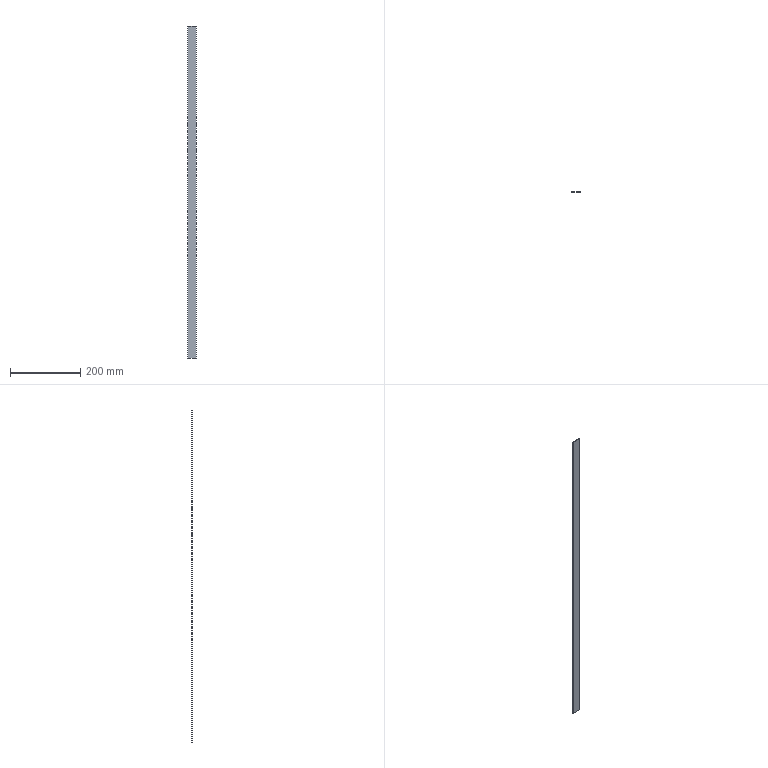Part | NX | features BREP 1 | 1 solid | 6 faces | box 24.5 x 0.5 x 943 mm | volume 11552 mm3 | plane 6
STEP:
#1=CARTESIAN_POINT('',(0.5,0.5,-471.5));
#2=VERTEX_POINT('',#1);
#3=CARTESIAN_POINT('',(25.,0.5,-471.5));
#4=VERTEX_POINT('',#3);
#5=CARTESIAN_POINT('',(0.,0.5,-471.5));
#6=DIRECTION('',(1.,0.,0.));
#7=VECTOR('',#6,1000.);
#8=LINE('',#5,#7);
#9=EDGE_CURVE('',#2,#4,#8,.T.);
#10=ORIENTED_EDGE('',*,*,#9,.F.);
#11=CARTESIAN_POINT('',(0.5,0.5,471.5));
#12=VERTEX_POINT('',#11);
#13=CARTESIAN_POINT('',(0.5,0.5,471.5));
#14=DIRECTION('',(0.,0.,-1.));
#15=VECTOR('',#14,1000.);
#16=LINE('',#13,#15);
#17=EDGE_CURVE('',#12,#2,#16,.T.);
#18=ORIENTED_EDGE('',*,*,#17,.F.);
#19=CARTESIAN_POINT('',(25.,0.5,471.5));
#20=VERTEX_POINT('',#19);
#21=CARTESIAN_POINT('',(0.,0.5,471.5));
#22=DIRECTION('',(-1.,0.,0.));
#23=VECTOR('',#22,1000.);
#24=LINE('',#21,#23);
#25=EDGE_CURVE('',#20,#12,#24,.T.);
#26=ORIENTED_EDGE('',*,*,#25,.F.);
#27=CARTESIAN_POINT('',(25.,0.5,471.5));
#28=DIRECTION('',(0.,0.,1.));
#29=VECTOR('',#28,1000.);
#30=LINE('',#27,#29);
#31=EDGE_CURVE('',#4,#20,#30,.T.);
#32=ORIENTED_EDGE('',*,*,#31,.F.);
#33=EDGE_LOOP('',(#10,#18,#26,#32));
#34=FACE_BOUND('',#33,.T.);
#35=CARTESIAN_POINT('',(0.,0.5,471.5));
#36=DIRECTION('',(0.,-1.,0.));
#37=DIRECTION('',(0.,0.,1.));
#38=AXIS2_PLACEMENT_3D('',#35,#36,#37);
#39=PLANE('',#38);
#40=ADVANCED_FACE('',(#34),#39,.F.);
#41=CARTESIAN_POINT('',(25.,0.,-471.5));
#42=VERTEX_POINT('',#41);
#43=CARTESIAN_POINT('',(25.,0.,471.5));
#44=VERTEX_POINT('',#43);
#45=CARTESIAN_POINT('',(25.,0.,471.5));
#46=DIRECTION('',(0.,0.,1.));
#47=VECTOR('',#46,1000.);
#48=LINE('',#45,#47);
#49=EDGE_CURVE('',#42,#44,#48,.T.);
#50=ORIENTED_EDGE('',*,*,#49,.F.);
#51=CARTESIAN_POINT('',(25.,0.5,-471.5));
#52=DIRECTION('',(0.,-1.,0.));
#53=VECTOR('',#52,1000.);
#54=LINE('',#51,#53);
#55=EDGE_CURVE('',#4,#42,#54,.T.);
#56=ORIENTED_EDGE('',*,*,#55,.F.);
#57=ORIENTED_EDGE('',*,*,#31,.T.);
#58=CARTESIAN_POINT('',(25.,0.5,471.5));
#59=DIRECTION('',(0.,1.,0.));
#60=VECTOR('',#59,1000.);
#61=LINE('',#58,#60);
#62=EDGE_CURVE('',#44,#20,#61,.T.);
#63=ORIENTED_EDGE('',*,*,#62,.F.);
#64=EDGE_LOOP('',(#50,#56,#57,#63));
#65=FACE_BOUND('',#64,.T.);
#66=CARTESIAN_POINT('',(25.,0.5,471.5));
#67=DIRECTION('',(-1.,0.,0.));
#68=DIRECTION('',(0.,0.,-1.));
#69=AXIS2_PLACEMENT_3D('',#66,#67,#68);
#70=PLANE('',#69);
#71=ADVANCED_FACE('',(#65),#70,.F.);
#72=ORIENTED_EDGE('',*,*,#9,.T.);
#73=ORIENTED_EDGE('',*,*,#55,.T.);
#74=CARTESIAN_POINT('',(0.5,0.,-471.5));
#75=VERTEX_POINT('',#74);
#76=CARTESIAN_POINT('',(0.52,0.,-471.5));
#77=DIRECTION('',(-1.,0.,0.));
#78=VECTOR('',#77,1000.);
#79=LINE('',#76,#78);
#80=EDGE_CURVE('',#42,#75,#79,.T.);
#81=ORIENTED_EDGE('',*,*,#80,.T.);
#82=CARTESIAN_POINT('',(0.5,0.52,-471.5));
#83=DIRECTION('',(0.,1.,0.));
#84=VECTOR('',#83,1000.);
#85=LINE('',#82,#84);
#86=EDGE_CURVE('',#75,#2,#85,.T.);
#87=ORIENTED_EDGE('',*,*,#86,.T.);
#88=EDGE_LOOP('',(#72,#73,#81,#87));
#89=FACE_BOUND('',#88,.T.);
#90=CARTESIAN_POINT('',(0.52,0.52,-471.5));
#91=DIRECTION('',(0.,0.,-1.));
#92=DIRECTION('',(1.,0.,0.));
#93=AXIS2_PLACEMENT_3D('',#90,#91,#92);
#94=PLANE('',#93);
#95=ADVANCED_FACE('',(#89),#94,.T.);
#96=CARTESIAN_POINT('',(0.5,0.,471.5));
#97=VERTEX_POINT('',#96);
#98=CARTESIAN_POINT('',(0.5,0.,0.));
#99=DIRECTION('',(0.,0.,1.));
#100=VECTOR('',#99,1000.);
#101=LINE('',#98,#100);
#102=EDGE_CURVE('',#75,#97,#101,.T.);
#103=ORIENTED_EDGE('',*,*,#102,.T.);
#104=CARTESIAN_POINT('',(0.5,0.,471.5));
#105=DIRECTION('',(0.,1.,0.));
#106=VECTOR('',#105,1000.);
#107=LINE('',#104,#106);
#108=EDGE_CURVE('',#97,#12,#107,.T.);
#109=ORIENTED_EDGE('',*,*,#108,.T.);
#110=ORIENTED_EDGE('',*,*,#17,.T.);
#111=ORIENTED_EDGE('',*,*,#86,.F.);
#112=EDGE_LOOP('',(#103,#109,#110,#111));
#113=FACE_BOUND('',#112,.T.);
#114=CARTESIAN_POINT('',(0.5,0.,0.));
#115=DIRECTION('',(-1.,0.,0.));
#116=DIRECTION('',(0.,0.,-1.));
#117=AXIS2_PLACEMENT_3D('',#114,#115,#116);
#118=PLANE('',#117);
#119=ADVANCED_FACE('',(#113),#118,.T.);
#120=CARTESIAN_POINT('',(0.5,0.,471.5));
#121=DIRECTION('',(1.,0.,0.));
#122=VECTOR('',#121,1000.);
#123=LINE('',#120,#122);
#124=EDGE_CURVE('',#97,#44,#123,.T.);
#125=ORIENTED_EDGE('',*,*,#124,.T.);
#126=ORIENTED_EDGE('',*,*,#62,.T.);
#127=ORIENTED_EDGE('',*,*,#25,.T.);
#128=ORIENTED_EDGE('',*,*,#108,.F.);
#129=EDGE_LOOP('',(#125,#126,#127,#128));
#130=FACE_BOUND('',#129,.T.);
#131=CARTESIAN_POINT('',(0.5,0.52,471.5));
#132=DIRECTION('',(0.,0.,1.));
#133=DIRECTION('',(-1.,0.,0.));
#134=AXIS2_PLACEMENT_3D('',#131,#132,#133);
#135=PLANE('',#134);
#136=ADVANCED_FACE('',(#130),#135,.T.);
#137=ORIENTED_EDGE('',*,*,#80,.F.);
#138=ORIENTED_EDGE('',*,*,#49,.T.);
#139=ORIENTED_EDGE('',*,*,#124,.F.);
#140=ORIENTED_EDGE('',*,*,#102,.F.);
#141=EDGE_LOOP('',(#137,#138,#139,#140));
#142=FACE_BOUND('',#141,.T.);
#143=CARTESIAN_POINT('',(0.,0.,471.5));
#144=DIRECTION('',(0.,-1.,0.));
#145=DIRECTION('',(0.,0.,1.));
#146=AXIS2_PLACEMENT_3D('',#143,#144,#145);
#147=PLANE('',#146);
#148=ADVANCED_FACE('',(#142),#147,.T.);
#149=CLOSED_SHELL('',(#40,#71,#95,#119,#136,#148));
#150=MANIFOLD_SOLID_BREP('',#149);
#151=(LENGTH_UNIT()NAMED_UNIT(*)SI_UNIT(.MILLI.,.METRE.));
#152=UNCERTAINTY_MEASURE_WITH_UNIT(LENGTH_MEASURE(0.00001),#151,'','');
#153=(NAMED_UNIT(*)PLANE_ANGLE_UNIT()SI_UNIT($,.RADIAN.));
#154=(NAMED_UNIT(*)SI_UNIT($,.STERADIAN.)SOLID_ANGLE_UNIT());
#155=(GEOMETRIC_REPRESENTATION_CONTEXT(3)GLOBAL_UNCERTAINTY_ASSIGNED_CONTEXT((#152))GLOBAL_UNIT_ASSIGNED_CONTEXT((#151,#153,#154))REPRESENTATION_CONTEXT('',''));
#156=ADVANCED_BREP_SHAPE_REPRESENTATION('',(#150),#155);